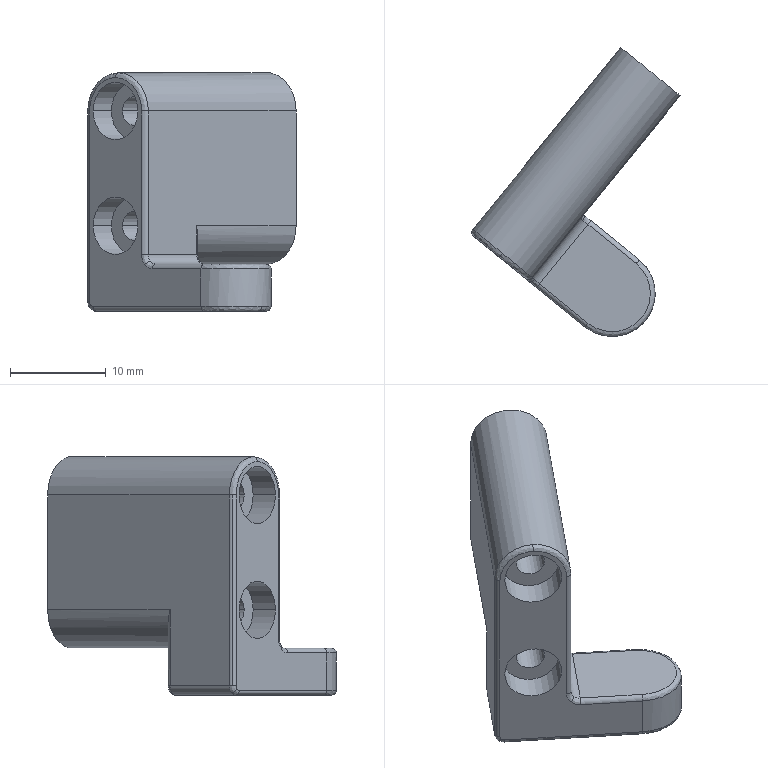Part | SolidWorks | features BaseBody 1 | 1 solid | 46 faces | box 21.777 x 30.184 x 24.936 mm | volume 4090 mm3 | cylinder 22 | spline 13 | plane 11 | commonest cylinder face diameters 1 x9 3 x4 6 x4 2 x2 8 x2 9 x1